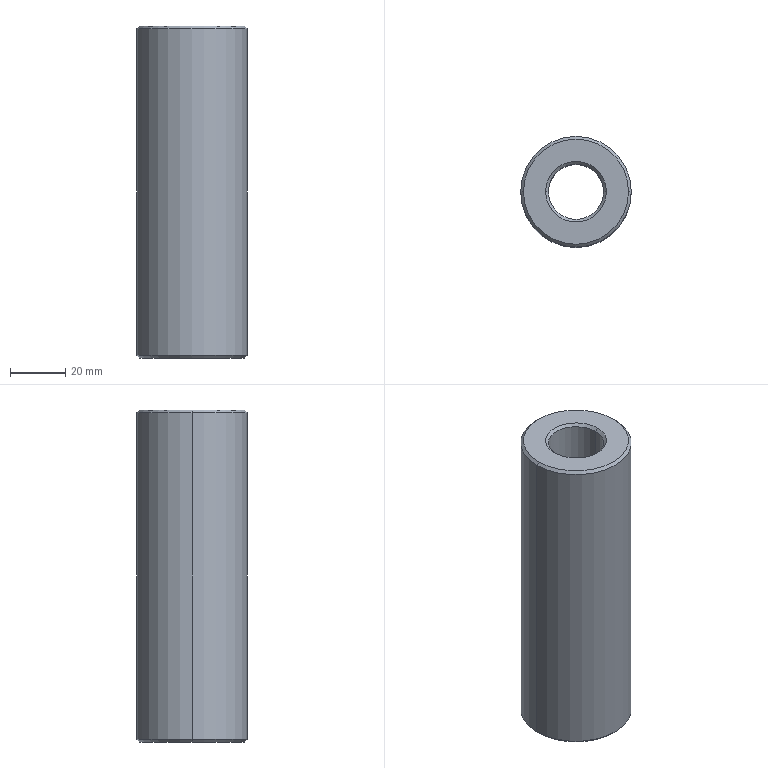Part | STEP file | BCC3 H14_7 | 1 solid | 14 faces | box 40 x 40 x 120 mm | volume 112909 mm3 | cone 8 | cylinder 4 | plane 2 | commonest cylinder face diameters 20 x2 40 x2
STEP:
#1=CARTESIAN_POINT('',(0.,0.,0.));
#2=DIRECTION('',(0.,0.,1.));
#3=DIRECTION('',(1.,0.,0.));
#4=AXIS2_PLACEMENT_3D('',#1,#2,#3);
#5=CARTESIAN_POINT('',(10.,0.,59.));
#6=VERTEX_POINT('',#5);
#7=CARTESIAN_POINT('',(11.,0.,60.));
#8=VERTEX_POINT('',#7);
#9=CARTESIAN_POINT('',(10.,0.,59.));
#10=DIRECTION('',(0.7071,0.,0.7071));
#11=VECTOR('',#10,1.);
#12=LINE('',#9,#11);
#13=CARTESIAN_POINT('',(0.,0.,59.));
#14=DIRECTION('',(0.,0.,1.));
#15=DIRECTION('',(1.,0.,0.));
#16=AXIS2_PLACEMENT_3D('',#13,#14,#15);
#17=CONICAL_SURFACE('',#16,10.,0.7854);
#18=CARTESIAN_POINT('',(6.283,0.));
#19=DIRECTION('',(0.,1.));
#20=VECTOR('',#19,1.);
#21=LINE('',#18,#20);
#22=(GEOMETRIC_REPRESENTATION_CONTEXT(2)PARAMETRIC_REPRESENTATION_CONTEXT()REPRESENTATION_CONTEXT('',''));
#23=DEFINITIONAL_REPRESENTATION('',(#21),#22);
#24=PCURVE('',#17,#23);
#25=CARTESIAN_POINT('',(0.,0.,59.));
#26=DIRECTION('',(0.,0.,1.));
#27=DIRECTION('',(1.,0.,0.));
#28=AXIS2_PLACEMENT_3D('',#25,#26,#27);
#29=CONICAL_SURFACE('',#28,10.,0.7854);
#30=CARTESIAN_POINT('',(0.,0.));
#31=DIRECTION('',(0.,1.));
#32=VECTOR('',#31,1.);
#33=LINE('',#30,#32);
#34=(GEOMETRIC_REPRESENTATION_CONTEXT(2)PARAMETRIC_REPRESENTATION_CONTEXT()REPRESENTATION_CONTEXT('',''));
#35=DEFINITIONAL_REPRESENTATION('',(#33),#34);
#36=PCURVE('',#29,#35);
#37=SURFACE_CURVE('',#12,(#24,#36),.PCURVE_S1.);
#38=EDGE_CURVE('',#6,#8,#37,.T.);
#39=ORIENTED_EDGE('',*,*,#38,.T.);
#40=CARTESIAN_POINT('',(-11.,0.,60.));
#41=VERTEX_POINT('',#40);
#42=CARTESIAN_POINT('',(0.,0.,60.));
#43=DIRECTION('',(0.,0.,-1.));
#44=DIRECTION('',(1.,0.,0.));
#45=AXIS2_PLACEMENT_3D('',#42,#43,#44);
#46=CIRCLE('',#45,11.);
#47=CARTESIAN_POINT('',(6.283,1.));
#48=DIRECTION('',(-1.,0.));
#49=VECTOR('',#48,1.);
#50=LINE('',#47,#49);
#51=(GEOMETRIC_REPRESENTATION_CONTEXT(2)PARAMETRIC_REPRESENTATION_CONTEXT()REPRESENTATION_CONTEXT('',''));
#52=DEFINITIONAL_REPRESENTATION('',(#50),#51);
#53=PCURVE('',#17,#52);
#54=CARTESIAN_POINT('',(0.,0.,60.));
#55=DIRECTION('',(0.,0.,1.));
#56=DIRECTION('',(1.,0.,0.));
#57=AXIS2_PLACEMENT_3D('',#54,#55,#56);
#58=PLANE('',#57);
#59=CARTESIAN_POINT('',(11.,0.));
#60=CARTESIAN_POINT('',(11.,-19.053));
#61=CARTESIAN_POINT('',(-5.5,-9.526));
#62=CARTESIAN_POINT('',(-22.,0.));
#63=CARTESIAN_POINT('',(-5.5,9.526));
#64=CARTESIAN_POINT('',(11.,19.053));
#65=CARTESIAN_POINT('',(11.,0.));
#66=(BOUNDED_CURVE()B_SPLINE_CURVE(2,(#59,#60,#61,#62,#63,#64,#65),.UNSPECIFIED.,.T.,.F.)B_SPLINE_CURVE_WITH_KNOTS((1,2,2,2,2,1),(-2.094,0.,2.094,4.189,6.283,8.378),.UNSPECIFIED.)CURVE()GEOMETRIC_REPRESENTATION_ITEM()RATIONAL_B_SPLINE_CURVE((1.,0.5,1.,0.5,1.,0.5,1.))REPRESENTATION_ITEM(''));
#67=(GEOMETRIC_REPRESENTATION_CONTEXT(2)PARAMETRIC_REPRESENTATION_CONTEXT()REPRESENTATION_CONTEXT('',''));
#68=DEFINITIONAL_REPRESENTATION('',(#66),#67);
#69=PCURVE('',#58,#68);
#70=SURFACE_CURVE('',#46,(#53,#69),.PCURVE_S1.);
#71=EDGE_CURVE('',#8,#41,#70,.T.);
#72=ORIENTED_EDGE('',*,*,#71,.T.);
#73=CARTESIAN_POINT('',(-10.,0.,59.));
#74=VERTEX_POINT('',#73);
#75=CARTESIAN_POINT('',(-10.,0.,59.));
#76=DIRECTION('',(-0.7071,0.,0.7071));
#77=VECTOR('',#76,1.);
#78=LINE('',#75,#77);
#79=CARTESIAN_POINT('',(3.142,0.));
#80=DIRECTION('',(0.,1.));
#81=VECTOR('',#80,1.);
#82=LINE('',#79,#81);
#83=(GEOMETRIC_REPRESENTATION_CONTEXT(2)PARAMETRIC_REPRESENTATION_CONTEXT()REPRESENTATION_CONTEXT('',''));
#84=DEFINITIONAL_REPRESENTATION('',(#82),#83);
#85=PCURVE('',#17,#84);
#86=CARTESIAN_POINT('',(3.142,0.));
#87=DIRECTION('',(0.,1.));
#88=VECTOR('',#87,1.);
#89=LINE('',#86,#88);
#90=(GEOMETRIC_REPRESENTATION_CONTEXT(2)PARAMETRIC_REPRESENTATION_CONTEXT()REPRESENTATION_CONTEXT('',''));
#91=DEFINITIONAL_REPRESENTATION('',(#89),#90);
#92=PCURVE('',#29,#91);
#93=SURFACE_CURVE('',#78,(#85,#92),.PCURVE_S1.);
#94=EDGE_CURVE('',#74,#41,#93,.T.);
#95=ORIENTED_EDGE('',*,*,#94,.F.);
#96=CARTESIAN_POINT('',(0.,0.,59.));
#97=DIRECTION('',(0.,0.,1.));
#98=DIRECTION('',(1.,0.,0.));
#99=AXIS2_PLACEMENT_3D('',#96,#97,#98);
#100=CIRCLE('',#99,10.);
#101=CARTESIAN_POINT('',(0.,0.));
#102=DIRECTION('',(1.,0.));
#103=VECTOR('',#102,1.);
#104=LINE('',#101,#103);
#105=(GEOMETRIC_REPRESENTATION_CONTEXT(2)PARAMETRIC_REPRESENTATION_CONTEXT()REPRESENTATION_CONTEXT('',''));
#106=DEFINITIONAL_REPRESENTATION('',(#104),#105);
#107=PCURVE('',#17,#106);
#108=CARTESIAN_POINT('',(0.,0.,60.));
#109=DIRECTION('',(0.,0.,-1.));
#110=DIRECTION('',(-1.,0.,0.));
#111=AXIS2_PLACEMENT_3D('',#108,#109,#110);
#112=CYLINDRICAL_SURFACE('',#111,10.);
#113=CARTESIAN_POINT('',(9.425,1.));
#114=DIRECTION('',(-1.,0.));
#115=VECTOR('',#114,1.);
#116=LINE('',#113,#115);
#117=(GEOMETRIC_REPRESENTATION_CONTEXT(2)PARAMETRIC_REPRESENTATION_CONTEXT()REPRESENTATION_CONTEXT('',''));
#118=DEFINITIONAL_REPRESENTATION('',(#116),#117);
#119=PCURVE('',#112,#118);
#120=SURFACE_CURVE('',#100,(#107,#119),.PCURVE_S1.);
#121=EDGE_CURVE('',#74,#6,#120,.T.);
#122=ORIENTED_EDGE('',*,*,#121,.T.);
#123=EDGE_LOOP('',(#39,#72,#95,#122));
#124=FACE_BOUND('',#123,.F.);
#125=ADVANCED_FACE('',(#124),#17,.F.);
#126=CARTESIAN_POINT('',(19.,0.,60.));
#127=VERTEX_POINT('',#126);
#128=CARTESIAN_POINT('',(-19.,0.,60.));
#129=VERTEX_POINT('',#128);
#130=CARTESIAN_POINT('',(0.,0.,60.));
#131=DIRECTION('',(0.,0.,1.));
#132=DIRECTION('',(1.,0.,0.));
#133=AXIS2_PLACEMENT_3D('',#130,#131,#132);
#134=CIRCLE('',#133,19.);
#135=CARTESIAN_POINT('',(0.,0.,60.));
#136=DIRECTION('',(0.,0.,-1.));
#137=DIRECTION('',(-1.,0.,0.));
#138=AXIS2_PLACEMENT_3D('',#135,#136,#137);
#139=CONICAL_SURFACE('',#138,19.,0.7854);
#140=CARTESIAN_POINT('',(3.142,0.));
#141=DIRECTION('',(-1.,0.));
#142=VECTOR('',#141,1.);
#143=LINE('',#140,#142);
#144=(GEOMETRIC_REPRESENTATION_CONTEXT(2)PARAMETRIC_REPRESENTATION_CONTEXT()REPRESENTATION_CONTEXT('',''));
#145=DEFINITIONAL_REPRESENTATION('',(#143),#144);
#146=PCURVE('',#139,#145);
#147=CARTESIAN_POINT('',(0.,0.));
#148=DIRECTION('',(1.,0.));
#149=AXIS2_PLACEMENT_2D('',#147,#148);
#150=CIRCLE('',#149,19.);
#151=(GEOMETRIC_REPRESENTATION_CONTEXT(2)PARAMETRIC_REPRESENTATION_CONTEXT()REPRESENTATION_CONTEXT('',''));
#152=DEFINITIONAL_REPRESENTATION('',(#150),#151);
#153=PCURVE('',#58,#152);
#154=SURFACE_CURVE('',#134,(#146,#153),.PCURVE_S1.);
#155=EDGE_CURVE('',#127,#129,#154,.T.);
#156=ORIENTED_EDGE('',*,*,#155,.F.);
#157=CARTESIAN_POINT('',(20.,0.,59.));
#158=VERTEX_POINT('',#157);
#159=CARTESIAN_POINT('',(19.,0.,60.));
#160=DIRECTION('',(0.7071,0.,-0.7071));
#161=VECTOR('',#160,1.);
#162=LINE('',#159,#161);
#163=CARTESIAN_POINT('',(3.142,0.));
#164=DIRECTION('',(0.,1.));
#165=VECTOR('',#164,1.);
#166=LINE('',#163,#165);
#167=(GEOMETRIC_REPRESENTATION_CONTEXT(2)PARAMETRIC_REPRESENTATION_CONTEXT()REPRESENTATION_CONTEXT('',''));
#168=DEFINITIONAL_REPRESENTATION('',(#166),#167);
#169=PCURVE('',#139,#168);
#170=CARTESIAN_POINT('',(0.,0.,60.));
#171=DIRECTION('',(0.,0.,-1.));
#172=DIRECTION('',(-1.,0.,0.));
#173=AXIS2_PLACEMENT_3D('',#170,#171,#172);
#174=CONICAL_SURFACE('',#173,19.,0.7854);
#175=CARTESIAN_POINT('',(3.142,0.));
#176=DIRECTION('',(0.,1.));
#177=VECTOR('',#176,1.);
#178=LINE('',#175,#177);
#179=(GEOMETRIC_REPRESENTATION_CONTEXT(2)PARAMETRIC_REPRESENTATION_CONTEXT()REPRESENTATION_CONTEXT('',''));
#180=DEFINITIONAL_REPRESENTATION('',(#178),#179);
#181=PCURVE('',#174,#180);
#182=SURFACE_CURVE('',#162,(#169,#181),.PCURVE_S1.);
#183=EDGE_CURVE('',#127,#158,#182,.T.);
#184=ORIENTED_EDGE('',*,*,#183,.T.);
#185=CARTESIAN_POINT('',(-20.,0.,59.));
#186=VERTEX_POINT('',#185);
#187=CARTESIAN_POINT('',(0.,0.,59.));
#188=DIRECTION('',(0.,0.,-1.));
#189=DIRECTION('',(1.,0.,0.));
#190=AXIS2_PLACEMENT_3D('',#187,#188,#189);
#191=CIRCLE('',#190,20.);
#192=CARTESIAN_POINT('',(-3.142,1.));
#193=DIRECTION('',(1.,0.));
#194=VECTOR('',#193,1.);
#195=LINE('',#192,#194);
#196=(GEOMETRIC_REPRESENTATION_CONTEXT(2)PARAMETRIC_REPRESENTATION_CONTEXT()REPRESENTATION_CONTEXT('',''));
#197=DEFINITIONAL_REPRESENTATION('',(#195),#196);
#198=PCURVE('',#139,#197);
#199=CARTESIAN_POINT('',(0.,0.,60.));
#200=DIRECTION('',(0.,0.,-1.));
#201=DIRECTION('',(-1.,0.,0.));
#202=AXIS2_PLACEMENT_3D('',#199,#200,#201);
#203=CYLINDRICAL_SURFACE('',#202,20.);
#204=CARTESIAN_POINT('',(-3.142,1.));
#205=DIRECTION('',(1.,0.));
#206=VECTOR('',#205,1.);
#207=LINE('',#204,#206);
#208=(GEOMETRIC_REPRESENTATION_CONTEXT(2)PARAMETRIC_REPRESENTATION_CONTEXT()REPRESENTATION_CONTEXT('',''));
#209=DEFINITIONAL_REPRESENTATION('',(#207),#208);
#210=PCURVE('',#203,#209);
#211=SURFACE_CURVE('',#191,(#198,#210),.PCURVE_S1.);
#212=EDGE_CURVE('',#186,#158,#211,.T.);
#213=ORIENTED_EDGE('',*,*,#212,.F.);
#214=CARTESIAN_POINT('',(-19.,0.,60.));
#215=DIRECTION('',(-0.7071,0.,-0.7071));
#216=VECTOR('',#215,1.);
#217=LINE('',#214,#216);
#218=CARTESIAN_POINT('',(0.,0.));
#219=DIRECTION('',(0.,1.));
#220=VECTOR('',#219,1.);
#221=LINE('',#218,#220);
#222=(GEOMETRIC_REPRESENTATION_CONTEXT(2)PARAMETRIC_REPRESENTATION_CONTEXT()REPRESENTATION_CONTEXT('',''));
#223=DEFINITIONAL_REPRESENTATION('',(#221),#222);
#224=PCURVE('',#139,#223);
#225=CARTESIAN_POINT('',(6.283,0.));
#226=DIRECTION('',(0.,1.));
#227=VECTOR('',#226,1.);
#228=LINE('',#225,#227);
#229=(GEOMETRIC_REPRESENTATION_CONTEXT(2)PARAMETRIC_REPRESENTATION_CONTEXT()REPRESENTATION_CONTEXT('',''));
#230=DEFINITIONAL_REPRESENTATION('',(#228),#229);
#231=PCURVE('',#174,#230);
#232=SURFACE_CURVE('',#217,(#224,#231),.PCURVE_S1.);
#233=EDGE_CURVE('',#129,#186,#232,.T.);
#234=ORIENTED_EDGE('',*,*,#233,.F.);
#235=EDGE_LOOP('',(#156,#184,#213,#234));
#236=FACE_BOUND('',#235,.T.);
#237=ADVANCED_FACE('',(#236),#139,.T.);
#238=CARTESIAN_POINT('',(-10.,0.,-59.));
#239=VERTEX_POINT('',#238);
#240=CARTESIAN_POINT('',(-11.,0.,-60.));
#241=VERTEX_POINT('',#240);
#242=CARTESIAN_POINT('',(-11.,0.,-60.));
#243=DIRECTION('',(-0.7071,0.,-0.7071));
#244=VECTOR('',#243,1.);
#245=LINE('',#242,#244);
#246=CARTESIAN_POINT('',(0.,0.,-60.));
#247=DIRECTION('',(0.,0.,-1.));
#248=DIRECTION('',(-1.,0.,0.));
#249=AXIS2_PLACEMENT_3D('',#246,#247,#248);
#250=CONICAL_SURFACE('',#249,11.,0.7854);
#251=CARTESIAN_POINT('',(6.283,0.));
#252=DIRECTION('',(0.,1.));
#253=VECTOR('',#252,1.);
#254=LINE('',#251,#253);
#255=(GEOMETRIC_REPRESENTATION_CONTEXT(2)PARAMETRIC_REPRESENTATION_CONTEXT()REPRESENTATION_CONTEXT('',''));
#256=DEFINITIONAL_REPRESENTATION('',(#254),#255);
#257=PCURVE('',#250,#256);
#258=CARTESIAN_POINT('',(0.,0.,-60.));
#259=DIRECTION('',(0.,0.,-1.));
#260=DIRECTION('',(-1.,0.,0.));
#261=AXIS2_PLACEMENT_3D('',#258,#259,#260);
#262=CONICAL_SURFACE('',#261,11.,0.7854);
#263=CARTESIAN_POINT('',(0.,0.));
#264=DIRECTION('',(0.,1.));
#265=VECTOR('',#264,1.);
#266=LINE('',#263,#265);
#267=(GEOMETRIC_REPRESENTATION_CONTEXT(2)PARAMETRIC_REPRESENTATION_CONTEXT()REPRESENTATION_CONTEXT('',''));
#268=DEFINITIONAL_REPRESENTATION('',(#266),#267);
#269=PCURVE('',#262,#268);
#270=SURFACE_CURVE('',#245,(#257,#269),.PCURVE_S1.);
#271=EDGE_CURVE('',#239,#241,#270,.T.);
#272=ORIENTED_EDGE('',*,*,#271,.T.);
#273=CARTESIAN_POINT('',(11.,0.,-60.));
#274=VERTEX_POINT('',#273);
#275=CARTESIAN_POINT('',(0.,0.,-60.));
#276=DIRECTION('',(0.,0.,1.));
#277=DIRECTION('',(1.,0.,0.));
#278=AXIS2_PLACEMENT_3D('',#275,#276,#277);
#279=CIRCLE('',#278,11.);
#280=CARTESIAN_POINT('',(9.425,0.));
#281=DIRECTION('',(-1.,0.));
#282=VECTOR('',#281,1.);
#283=LINE('',#280,#282);
#284=(GEOMETRIC_REPRESENTATION_CONTEXT(2)PARAMETRIC_REPRESENTATION_CONTEXT()REPRESENTATION_CONTEXT('',''));
#285=DEFINITIONAL_REPRESENTATION('',(#283),#284);
#286=PCURVE('',#250,#285);
#287=CARTESIAN_POINT('',(0.,0.,-60.));
#288=DIRECTION('',(0.,0.,1.));
#289=DIRECTION('',(1.,0.,0.));
#290=AXIS2_PLACEMENT_3D('',#287,#288,#289);
#291=PLANE('',#290);
#292=CARTESIAN_POINT('',(0.,0.));
#293=DIRECTION('',(1.,0.));
#294=AXIS2_PLACEMENT_2D('',#292,#293);
#295=CIRCLE('',#294,11.);
#296=(GEOMETRIC_REPRESENTATION_CONTEXT(2)PARAMETRIC_REPRESENTATION_CONTEXT()REPRESENTATION_CONTEXT('',''));
#297=DEFINITIONAL_REPRESENTATION('',(#295),#296);
#298=PCURVE('',#291,#297);
#299=SURFACE_CURVE('',#279,(#286,#298),.PCURVE_S1.);
#300=EDGE_CURVE('',#241,#274,#299,.T.);
#301=ORIENTED_EDGE('',*,*,#300,.T.);
#302=CARTESIAN_POINT('',(10.,0.,-59.));
#303=VERTEX_POINT('',#302);
#304=CARTESIAN_POINT('',(11.,0.,-60.));
#305=DIRECTION('',(0.7071,0.,-0.7071));
#306=VECTOR('',#305,1.);
#307=LINE('',#304,#306);
#308=CARTESIAN_POINT('',(3.142,0.));
#309=DIRECTION('',(0.,1.));
#310=VECTOR('',#309,1.);
#311=LINE('',#308,#310);
#312=(GEOMETRIC_REPRESENTATION_CONTEXT(2)PARAMETRIC_REPRESENTATION_CONTEXT()REPRESENTATION_CONTEXT('',''));
#313=DEFINITIONAL_REPRESENTATION('',(#311),#312);
#314=PCURVE('',#250,#313);
#315=CARTESIAN_POINT('',(3.142,0.));
#316=DIRECTION('',(0.,1.));
#317=VECTOR('',#316,1.);
#318=LINE('',#315,#317);
#319=(GEOMETRIC_REPRESENTATION_CONTEXT(2)PARAMETRIC_REPRESENTATION_CONTEXT()REPRESENTATION_CONTEXT('',''));
#320=DEFINITIONAL_REPRESENTATION('',(#318),#319);
#321=PCURVE('',#262,#320);
#322=SURFACE_CURVE('',#307,(#314,#321),.PCURVE_S1.);
#323=EDGE_CURVE('',#303,#274,#322,.T.);
#324=ORIENTED_EDGE('',*,*,#323,.F.);
#325=CARTESIAN_POINT('',(0.,0.,-59.));
#326=DIRECTION('',(0.,0.,-1.));
#327=DIRECTION('',(1.,0.,0.));
#328=AXIS2_PLACEMENT_3D('',#325,#326,#327);
#329=CIRCLE('',#328,10.);
#330=CARTESIAN_POINT('',(3.142,-1.));
#331=DIRECTION('',(1.,0.));
#332=VECTOR('',#331,1.);
#333=LINE('',#330,#332);
#334=(GEOMETRIC_REPRESENTATION_CONTEXT(2)PARAMETRIC_REPRESENTATION_CONTEXT()REPRESENTATION_CONTEXT('',''));
#335=DEFINITIONAL_REPRESENTATION('',(#333),#334);
#336=PCURVE('',#250,#335);
#337=CARTESIAN_POINT('',(3.142,119.));
#338=DIRECTION('',(1.,0.));
#339=VECTOR('',#338,1.);
#340=LINE('',#337,#339);
#341=(GEOMETRIC_REPRESENTATION_CONTEXT(2)PARAMETRIC_REPRESENTATION_CONTEXT()REPRESENTATION_CONTEXT('',''));
#342=DEFINITIONAL_REPRESENTATION('',(#340),#341);
#343=PCURVE('',#112,#342);
#344=SURFACE_CURVE('',#329,(#336,#343),.PCURVE_S1.);
#345=EDGE_CURVE('',#303,#239,#344,.T.);
#346=ORIENTED_EDGE('',*,*,#345,.T.);
#347=EDGE_LOOP('',(#272,#301,#324,#346));
#348=FACE_BOUND('',#347,.F.);
#349=ADVANCED_FACE('',(#348),#250,.F.);
#350=CARTESIAN_POINT('',(-19.,0.,-60.));
#351=VERTEX_POINT('',#350);
#352=CARTESIAN_POINT('',(19.,0.,-60.));
#353=VERTEX_POINT('',#352);
#354=CARTESIAN_POINT('',(0.,0.,-60.));
#355=DIRECTION('',(0.,0.,-1.));
#356=DIRECTION('',(1.,0.,0.));
#357=AXIS2_PLACEMENT_3D('',#354,#355,#356);
#358=CIRCLE('',#357,19.);
#359=CARTESIAN_POINT('',(0.,0.,-59.));
#360=DIRECTION('',(0.,0.,1.));
#361=DIRECTION('',(1.,0.,0.));
#362=AXIS2_PLACEMENT_3D('',#359,#360,#361);
#363=CONICAL_SURFACE('',#362,20.,0.7854);
#364=CARTESIAN_POINT('',(6.283,-1.));
#365=DIRECTION('',(-1.,0.));
#366=VECTOR('',#365,1.);
#367=LINE('',#364,#366);
#368=(GEOMETRIC_REPRESENTATION_CONTEXT(2)PARAMETRIC_REPRESENTATION_CONTEXT()REPRESENTATION_CONTEXT('',''));
#369=DEFINITIONAL_REPRESENTATION('',(#367),#368);
#370=PCURVE('',#363,#369);
#371=CARTESIAN_POINT('',(19.,0.));
#372=CARTESIAN_POINT('',(19.,-32.909));
#373=CARTESIAN_POINT('',(-9.5,-16.454));
#374=CARTESIAN_POINT('',(-38.,0.));
#375=CARTESIAN_POINT('',(-9.5,16.454));
#376=CARTESIAN_POINT('',(19.,32.909));
#377=CARTESIAN_POINT('',(19.,0.));
#378=(BOUNDED_CURVE()B_SPLINE_CURVE(2,(#371,#372,#373,#374,#375,#376,#377),.UNSPECIFIED.,.T.,.F.)B_SPLINE_CURVE_WITH_KNOTS((1,2,2,2,2,1),(-2.094,0.,2.094,4.189,6.283,8.378),.UNSPECIFIED.)CURVE()GEOMETRIC_REPRESENTATION_ITEM()RATIONAL_B_SPLINE_CURVE((1.,0.5,1.,0.5,1.,0.5,1.))REPRESENTATION_ITEM(''));
#379=(GEOMETRIC_REPRESENTATION_CONTEXT(2)PARAMETRIC_REPRESENTATION_CONTEXT()REPRESENTATION_CONTEXT('',''));
#380=DEFINITIONAL_REPRESENTATION('',(#378),#379);
#381=PCURVE('',#291,#380);
#382=SURFACE_CURVE('',#358,(#370,#381),.PCURVE_S1.);
#383=EDGE_CURVE('',#351,#353,#382,.T.);
#384=ORIENTED_EDGE('',*,*,#383,.F.);
#385=CARTESIAN_POINT('',(-20.,0.,-59.));
#386=VERTEX_POINT('',#385);
#387=CARTESIAN_POINT('',(-20.,0.,-59.));
#388=DIRECTION('',(-0.7071,0.,0.7071));
#389=VECTOR('',#388,1.);
#390=LINE('',#387,#389);
#391=CARTESIAN_POINT('',(3.142,0.));
#392=DIRECTION('',(0.,1.));
#393=VECTOR('',#392,1.);
#394=LINE('',#391,#393);
#395=(GEOMETRIC_REPRESENTATION_CONTEXT(2)PARAMETRIC_REPRESENTATION_CONTEXT()REPRESENTATION_CONTEXT('',''));
#396=DEFINITIONAL_REPRESENTATION('',(#394),#395);
#397=PCURVE('',#363,#396);
#398=CARTESIAN_POINT('',(0.,0.,-59.));
#399=DIRECTION('',(0.,0.,1.));
#400=DIRECTION('',(1.,0.,0.));
#401=AXIS2_PLACEMENT_3D('',#398,#399,#400);
#402=CONICAL_SURFACE('',#401,20.,0.7854);
#403=CARTESIAN_POINT('',(3.142,0.));
#404=DIRECTION('',(0.,1.));
#405=VECTOR('',#404,1.);
#406=LINE('',#403,#405);
#407=(GEOMETRIC_REPRESENTATION_CONTEXT(2)PARAMETRIC_REPRESENTATION_CONTEXT()REPRESENTATION_CONTEXT('',''));
#408=DEFINITIONAL_REPRESENTATION('',(#406),#407);
#409=PCURVE('',#402,#408);
#410=SURFACE_CURVE('',#390,(#397,#409),.PCURVE_S1.);
#411=EDGE_CURVE('',#351,#386,#410,.T.);
#412=ORIENTED_EDGE('',*,*,#411,.T.);
#413=CARTESIAN_POINT('',(20.,0.,-59.));
#414=VERTEX_POINT('',#413);
#415=CARTESIAN_POINT('',(0.,0.,-59.));
#416=DIRECTION('',(0.,0.,1.));
#417=DIRECTION('',(1.,0.,0.));
#418=AXIS2_PLACEMENT_3D('',#415,#416,#417);
#419=CIRCLE('',#418,20.);
#420=CARTESIAN_POINT('',(0.,0.));
#421=DIRECTION('',(1.,0.));
#422=VECTOR('',#421,1.);
#423=LINE('',#420,#422);
#424=(GEOMETRIC_REPRESENTATION_CONTEXT(2)PARAMETRIC_REPRESENTATION_CONTEXT()REPRESENTATION_CONTEXT('',''));
#425=DEFINITIONAL_REPRESENTATION('',(#423),#424);
#426=PCURVE('',#363,#425);
#427=CARTESIAN_POINT('',(3.142,119.));
#428=DIRECTION('',(-1.,0.));
#429=VECTOR('',#428,1.);
#430=LINE('',#427,#429);
#431=(GEOMETRIC_REPRESENTATION_CONTEXT(2)PARAMETRIC_REPRESENTATION_CONTEXT()REPRESENTATION_CONTEXT('',''));
#432=DEFINITIONAL_REPRESENTATION('',(#430),#431);
#433=PCURVE('',#203,#432);
#434=SURFACE_CURVE('',#419,(#426,#433),.PCURVE_S1.);
#435=EDGE_CURVE('',#414,#386,#434,.T.);
#436=ORIENTED_EDGE('',*,*,#435,.F.);
#437=CARTESIAN_POINT('',(20.,0.,-59.));
#438=DIRECTION('',(0.7071,0.,0.7071));
#439=VECTOR('',#438,1.);
#440=LINE('',#437,#439);
#441=CARTESIAN_POINT('',(0.,0.));
#442=DIRECTION('',(0.,1.));
#443=VECTOR('',#442,1.);
#444=LINE('',#441,#443);
#445=(GEOMETRIC_REPRESENTATION_CONTEXT(2)PARAMETRIC_REPRESENTATION_CONTEXT()REPRESENTATION_CONTEXT('',''));
#446=DEFINITIONAL_REPRESENTATION('',(#444),#445);
#447=PCURVE('',#363,#446);
#448=CARTESIAN_POINT('',(6.283,0.));
#449=DIRECTION('',(0.,1.));
#450=VECTOR('',#449,1.);
#451=LINE('',#448,#450);
#452=(GEOMETRIC_REPRESENTATION_CONTEXT(2)PARAMETRIC_REPRESENTATION_CONTEXT()REPRESENTATION_CONTEXT('',''));
#453=DEFINITIONAL_REPRESENTATION('',(#451),#452);
#454=PCURVE('',#402,#453);
#455=SURFACE_CURVE('',#440,(#447,#454),.PCURVE_S1.);
#456=EDGE_CURVE('',#353,#414,#455,.T.);
#457=ORIENTED_EDGE('',*,*,#456,.F.);
#458=EDGE_LOOP('',(#384,#412,#436,#457));
#459=FACE_BOUND('',#458,.T.);
#460=ADVANCED_FACE('',(#459),#363,.T.);
#461=CARTESIAN_POINT('',(-10.,0.,60.));
#462=DIRECTION('',(0.,0.,-1.));
#463=VECTOR('',#462,1.);
#464=LINE('',#461,#463);
#465=CARTESIAN_POINT('',(6.283,0.));
#466=DIRECTION('',(0.,1.));
#467=VECTOR('',#466,1.);
#468=LINE('',#465,#467);
#469=(GEOMETRIC_REPRESENTATION_CONTEXT(2)PARAMETRIC_REPRESENTATION_CONTEXT()REPRESENTATION_CONTEXT('',''));
#470=DEFINITIONAL_REPRESENTATION('',(#468),#469);
#471=PCURVE('',#112,#470);
#472=CARTESIAN_POINT('',(0.,0.,60.));
#473=DIRECTION('',(0.,0.,-1.));
#474=DIRECTION('',(-1.,0.,0.));
#475=AXIS2_PLACEMENT_3D('',#472,#473,#474);
#476=CYLINDRICAL_SURFACE('',#475,10.);
#477=CARTESIAN_POINT('',(0.,0.));
#478=DIRECTION('',(0.,1.));
#479=VECTOR('',#478,1.);
#480=LINE('',#477,#479);
#481=(GEOMETRIC_REPRESENTATION_CONTEXT(2)PARAMETRIC_REPRESENTATION_CONTEXT()REPRESENTATION_CONTEXT('',''));
#482=DEFINITIONAL_REPRESENTATION('',(#480),#481);
#483=PCURVE('',#476,#482);
#484=SURFACE_CURVE('',#464,(#471,#483),.PCURVE_S1.);
#485=EDGE_CURVE('',#74,#239,#484,.T.);
#486=ORIENTED_EDGE('',*,*,#485,.T.);
#487=ORIENTED_EDGE('',*,*,#345,.F.);
#488=CARTESIAN_POINT('',(10.,0.,60.));
#489=DIRECTION('',(0.,0.,-1.));
#490=VECTOR('',#489,1.);
#491=LINE('',#488,#490);
#492=CARTESIAN_POINT('',(3.142,0.));
#493=DIRECTION('',(0.,1.));
#494=VECTOR('',#493,1.);
#495=LINE('',#492,#494);
#496=(GEOMETRIC_REPRESENTATION_CONTEXT(2)PARAMETRIC_REPRESENTATION_CONTEXT()REPRESENTATION_CONTEXT('',''));
#497=DEFINITIONAL_REPRESENTATION('',(#495),#496);
#498=PCURVE('',#112,#497);
#499=CARTESIAN_POINT('',(3.142,0.));
#500=DIRECTION('',(0.,1.));
#501=VECTOR('',#500,1.);
#502=LINE('',#499,#501);
#503=(GEOMETRIC_REPRESENTATION_CONTEXT(2)PARAMETRIC_REPRESENTATION_CONTEXT()REPRESENTATION_CONTEXT('',''));
#504=DEFINITIONAL_REPRESENTATION('',(#502),#503);
#505=PCURVE('',#476,#504);
#506=SURFACE_CURVE('',#491,(#498,#505),.PCURVE_S1.);
#507=EDGE_CURVE('',#6,#303,#506,.T.);
#508=ORIENTED_EDGE('',*,*,#507,.F.);
#509=ORIENTED_EDGE('',*,*,#121,.F.);
#510=EDGE_LOOP('',(#486,#487,#508,#509));
#511=FACE_BOUND('',#510,.F.);
#512=ADVANCED_FACE('',(#511),#112,.F.);
#513=ORIENTED_EDGE('',*,*,#212,.T.);
#514=CARTESIAN_POINT('',(20.,0.,60.));
#515=DIRECTION('',(0.,0.,-1.));
#516=VECTOR('',#515,1.);
#517=LINE('',#514,#516);
#518=CARTESIAN_POINT('',(3.142,0.));
#519=DIRECTION('',(0.,1.));
#520=VECTOR('',#519,1.);
#521=LINE('',#518,#520);
#522=(GEOMETRIC_REPRESENTATION_CONTEXT(2)PARAMETRIC_REPRESENTATION_CONTEXT()REPRESENTATION_CONTEXT('',''));
#523=DEFINITIONAL_REPRESENTATION('',(#521),#522);
#524=PCURVE('',#203,#523);
#525=CARTESIAN_POINT('',(0.,0.,60.));
#526=DIRECTION('',(0.,0.,-1.));
#527=DIRECTION('',(-1.,0.,0.));
#528=AXIS2_PLACEMENT_3D('',#525,#526,#527);
#529=CYLINDRICAL_SURFACE('',#528,20.);
#530=CARTESIAN_POINT('',(3.142,0.));
#531=DIRECTION('',(0.,1.));
#532=VECTOR('',#531,1.);
#533=LINE('',#530,#532);
#534=(GEOMETRIC_REPRESENTATION_CONTEXT(2)PARAMETRIC_REPRESENTATION_CONTEXT()REPRESENTATION_CONTEXT('',''));
#535=DEFINITIONAL_REPRESENTATION('',(#533),#534);
#536=PCURVE('',#529,#535);
#537=SURFACE_CURVE('',#517,(#524,#536),.PCURVE_S1.);
#538=EDGE_CURVE('',#158,#414,#537,.T.);
#539=ORIENTED_EDGE('',*,*,#538,.T.);
#540=ORIENTED_EDGE('',*,*,#435,.T.);
#541=CARTESIAN_POINT('',(-20.,0.,60.));
#542=DIRECTION('',(0.,0.,-1.));
#543=VECTOR('',#542,1.);
#544=LINE('',#541,#543);
#545=CARTESIAN_POINT('',(0.,0.));
#546=DIRECTION('',(0.,1.));
#547=VECTOR('',#546,1.);
#548=LINE('',#545,#547);
#549=(GEOMETRIC_REPRESENTATION_CONTEXT(2)PARAMETRIC_REPRESENTATION_CONTEXT()REPRESENTATION_CONTEXT('',''));
#550=DEFINITIONAL_REPRESENTATION('',(#548),#549);
#551=PCURVE('',#203,#550);
#552=CARTESIAN_POINT('',(6.283,0.));
#553=DIRECTION('',(0.,1.));
#554=VECTOR('',#553,1.);
#555=LINE('',#552,#554);
#556=(GEOMETRIC_REPRESENTATION_CONTEXT(2)PARAMETRIC_REPRESENTATION_CONTEXT()REPRESENTATION_CONTEXT('',''));
#557=DEFINITIONAL_REPRESENTATION('',(#555),#556);
#558=PCURVE('',#529,#557);
#559=SURFACE_CURVE('',#544,(#551,#558),.PCURVE_S1.);
#560=EDGE_CURVE('',#186,#386,#559,.T.);
#561=ORIENTED_EDGE('',*,*,#560,.F.);
#562=EDGE_LOOP('',(#513,#539,#540,#561));
#563=FACE_BOUND('',#562,.T.);
#564=ADVANCED_FACE('',(#563),#203,.T.);
#565=CARTESIAN_POINT('',(0.,0.,60.));
#566=DIRECTION('',(0.,0.,1.));
#567=DIRECTION('',(1.,0.,0.));
#568=AXIS2_PLACEMENT_3D('',#565,#566,#567);
#569=CIRCLE('',#568,19.);
#570=CARTESIAN_POINT('',(0.,0.));
#571=DIRECTION('',(1.,0.));
#572=AXIS2_PLACEMENT_2D('',#570,#571);
#573=CIRCLE('',#572,19.);
#574=(GEOMETRIC_REPRESENTATION_CONTEXT(2)PARAMETRIC_REPRESENTATION_CONTEXT()REPRESENTATION_CONTEXT('',''));
#575=DEFINITIONAL_REPRESENTATION('',(#573),#574);
#576=PCURVE('',#58,#575);
#577=CARTESIAN_POINT('',(9.425,0.));
#578=DIRECTION('',(-1.,0.));
#579=VECTOR('',#578,1.);
#580=LINE('',#577,#579);
#581=(GEOMETRIC_REPRESENTATION_CONTEXT(2)PARAMETRIC_REPRESENTATION_CONTEXT()REPRESENTATION_CONTEXT('',''));
#582=DEFINITIONAL_REPRESENTATION('',(#580),#581);
#583=PCURVE('',#174,#582);
#584=SURFACE_CURVE('',#569,(#576,#583),.PCURVE_S1.);
#585=EDGE_CURVE('',#129,#127,#584,.T.);
#586=ORIENTED_EDGE('',*,*,#585,.T.);
#587=ORIENTED_EDGE('',*,*,#155,.T.);
#588=EDGE_LOOP('',(#586,#587));
#589=FACE_BOUND('',#588,.T.);
#590=ORIENTED_EDGE('',*,*,#71,.T.);
#591=CARTESIAN_POINT('',(0.,0.,60.));
#592=DIRECTION('',(0.,0.,-1.));
#593=DIRECTION('',(1.,0.,0.));
#594=AXIS2_PLACEMENT_3D('',#591,#592,#593);
#595=CIRCLE('',#594,11.);
#596=CARTESIAN_POINT('',(11.,0.));
#597=CARTESIAN_POINT('',(11.,-19.053));
#598=CARTESIAN_POINT('',(-5.5,-9.526));
#599=CARTESIAN_POINT('',(-22.,0.));
#600=CARTESIAN_POINT('',(-5.5,9.526));
#601=CARTESIAN_POINT('',(11.,19.053));
#602=CARTESIAN_POINT('',(11.,0.));
#603=(BOUNDED_CURVE()B_SPLINE_CURVE(2,(#596,#597,#598,#599,#600,#601,#602),.UNSPECIFIED.,.T.,.F.)B_SPLINE_CURVE_WITH_KNOTS((1,2,2,2,2,1),(-2.094,0.,2.094,4.189,6.283,8.378),.UNSPECIFIED.)CURVE()GEOMETRIC_REPRESENTATION_ITEM()RATIONAL_B_SPLINE_CURVE((1.,0.5,1.,0.5,1.,0.5,1.))REPRESENTATION_ITEM(''));
#604=(GEOMETRIC_REPRESENTATION_CONTEXT(2)PARAMETRIC_REPRESENTATION_CONTEXT()REPRESENTATION_CONTEXT('',''));
#605=DEFINITIONAL_REPRESENTATION('',(#603),#604);
#606=PCURVE('',#58,#605);
#607=CARTESIAN_POINT('',(6.283,1.));
#608=DIRECTION('',(-1.,0.));
#609=VECTOR('',#608,1.);
#610=LINE('',#607,#609);
#611=(GEOMETRIC_REPRESENTATION_CONTEXT(2)PARAMETRIC_REPRESENTATION_CONTEXT()REPRESENTATION_CONTEXT('',''));
#612=DEFINITIONAL_REPRESENTATION('',(#610),#611);
#613=PCURVE('',#29,#612);
#614=SURFACE_CURVE('',#595,(#606,#613),.PCURVE_S1.);
#615=EDGE_CURVE('',#41,#8,#614,.T.);
#616=ORIENTED_EDGE('',*,*,#615,.T.);
#617=EDGE_LOOP('',(#590,#616));
#618=FACE_BOUND('',#617,.T.);
#619=ADVANCED_FACE('',(#589,#618),#58,.T.);
#620=CARTESIAN_POINT('',(0.,0.,-60.));
#621=DIRECTION('',(0.,0.,-1.));
#622=DIRECTION('',(1.,0.,0.));
#623=AXIS2_PLACEMENT_3D('',#620,#621,#622);
#624=CIRCLE('',#623,19.);
#625=CARTESIAN_POINT('',(19.,0.));
#626=CARTESIAN_POINT('',(19.,-32.909));
#627=CARTESIAN_POINT('',(-9.5,-16.454));
#628=CARTESIAN_POINT('',(-38.,0.));
#629=CARTESIAN_POINT('',(-9.5,16.454));
#630=CARTESIAN_POINT('',(19.,32.909));
#631=CARTESIAN_POINT('',(19.,0.));
#632=(BOUNDED_CURVE()B_SPLINE_CURVE(2,(#625,#626,#627,#628,#629,#630,#631),.UNSPECIFIED.,.T.,.F.)B_SPLINE_CURVE_WITH_KNOTS((1,2,2,2,2,1),(-2.094,0.,2.094,4.189,6.283,8.378),.UNSPECIFIED.)CURVE()GEOMETRIC_REPRESENTATION_ITEM()RATIONAL_B_SPLINE_CURVE((1.,0.5,1.,0.5,1.,0.5,1.))REPRESENTATION_ITEM(''));
#633=(GEOMETRIC_REPRESENTATION_CONTEXT(2)PARAMETRIC_REPRESENTATION_CONTEXT()REPRESENTATION_CONTEXT('',''));
#634=DEFINITIONAL_REPRESENTATION('',(#632),#633);
#635=PCURVE('',#291,#634);
#636=CARTESIAN_POINT('',(6.283,-1.));
#637=DIRECTION('',(-1.,0.));
#638=VECTOR('',#637,1.);
#639=LINE('',#636,#638);
#640=(GEOMETRIC_REPRESENTATION_CONTEXT(2)PARAMETRIC_REPRESENTATION_CONTEXT()REPRESENTATION_CONTEXT('',''));
#641=DEFINITIONAL_REPRESENTATION('',(#639),#640);
#642=PCURVE('',#402,#641);
#643=SURFACE_CURVE('',#624,(#635,#642),.PCURVE_S1.);
#644=EDGE_CURVE('',#353,#351,#643,.T.);
#645=ORIENTED_EDGE('',*,*,#644,.T.);
#646=ORIENTED_EDGE('',*,*,#383,.T.);
#647=EDGE_LOOP('',(#645,#646));
#648=FACE_BOUND('',#647,.T.);
#649=ORIENTED_EDGE('',*,*,#300,.T.);
#650=CARTESIAN_POINT('',(0.,0.,-60.));
#651=DIRECTION('',(0.,0.,1.));
#652=DIRECTION('',(1.,0.,0.));
#653=AXIS2_PLACEMENT_3D('',#650,#651,#652);
#654=CIRCLE('',#653,11.);
#655=CARTESIAN_POINT('',(0.,0.));
#656=DIRECTION('',(1.,0.));
#657=AXIS2_PLACEMENT_2D('',#655,#656);
#658=CIRCLE('',#657,11.);
#659=(GEOMETRIC_REPRESENTATION_CONTEXT(2)PARAMETRIC_REPRESENTATION_CONTEXT()REPRESENTATION_CONTEXT('',''));
#660=DEFINITIONAL_REPRESENTATION('',(#658),#659);
#661=PCURVE('',#291,#660);
#662=CARTESIAN_POINT('',(3.142,0.));
#663=DIRECTION('',(-1.,0.));
#664=VECTOR('',#663,1.);
#665=LINE('',#662,#664);
#666=(GEOMETRIC_REPRESENTATION_CONTEXT(2)PARAMETRIC_REPRESENTATION_CONTEXT()REPRESENTATION_CONTEXT('',''));
#667=DEFINITIONAL_REPRESENTATION('',(#665),#666);
#668=PCURVE('',#262,#667);
#669=SURFACE_CURVE('',#654,(#661,#668),.PCURVE_S1.);
#670=EDGE_CURVE('',#274,#241,#669,.T.);
#671=ORIENTED_EDGE('',*,*,#670,.T.);
#672=EDGE_LOOP('',(#649,#671));
#673=FACE_BOUND('',#672,.T.);
#674=ADVANCED_FACE('',(#648,#673),#291,.F.);
#675=ORIENTED_EDGE('',*,*,#538,.F.);
#676=CARTESIAN_POINT('',(0.,0.,59.));
#677=DIRECTION('',(0.,0.,-1.));
#678=DIRECTION('',(1.,0.,0.));
#679=AXIS2_PLACEMENT_3D('',#676,#677,#678);
#680=CIRCLE('',#679,20.);
#681=CARTESIAN_POINT('',(3.142,1.));
#682=DIRECTION('',(1.,0.));
#683=VECTOR('',#682,1.);
#684=LINE('',#681,#683);
#685=(GEOMETRIC_REPRESENTATION_CONTEXT(2)PARAMETRIC_REPRESENTATION_CONTEXT()REPRESENTATION_CONTEXT('',''));
#686=DEFINITIONAL_REPRESENTATION('',(#684),#685);
#687=PCURVE('',#529,#686);
#688=CARTESIAN_POINT('',(3.142,1.));
#689=DIRECTION('',(1.,0.));
#690=VECTOR('',#689,1.);
#691=LINE('',#688,#690);
#692=(GEOMETRIC_REPRESENTATION_CONTEXT(2)PARAMETRIC_REPRESENTATION_CONTEXT()REPRESENTATION_CONTEXT('',''));
#693=DEFINITIONAL_REPRESENTATION('',(#691),#692);
#694=PCURVE('',#174,#693);
#695=SURFACE_CURVE('',#680,(#687,#694),.PCURVE_S1.);
#696=EDGE_CURVE('',#158,#186,#695,.T.);
#697=ORIENTED_EDGE('',*,*,#696,.T.);
#698=ORIENTED_EDGE('',*,*,#560,.T.);
#699=CARTESIAN_POINT('',(0.,0.,-59.));
#700=DIRECTION('',(0.,0.,1.));
#701=DIRECTION('',(1.,0.,0.));
#702=AXIS2_PLACEMENT_3D('',#699,#700,#701);
#703=CIRCLE('',#702,20.);
#704=CARTESIAN_POINT('',(9.425,119.));
#705=DIRECTION('',(-1.,0.));
#706=VECTOR('',#705,1.);
#707=LINE('',#704,#706);
#708=(GEOMETRIC_REPRESENTATION_CONTEXT(2)PARAMETRIC_REPRESENTATION_CONTEXT()REPRESENTATION_CONTEXT('',''));
#709=DEFINITIONAL_REPRESENTATION('',(#707),#708);
#710=PCURVE('',#529,#709);
#711=CARTESIAN_POINT('',(0.,0.));
#712=DIRECTION('',(1.,0.));
#713=VECTOR('',#712,1.);
#714=LINE('',#711,#713);
#715=(GEOMETRIC_REPRESENTATION_CONTEXT(2)PARAMETRIC_REPRESENTATION_CONTEXT()REPRESENTATION_CONTEXT('',''));
#716=DEFINITIONAL_REPRESENTATION('',(#714),#715);
#717=PCURVE('',#402,#716);
#718=SURFACE_CURVE('',#703,(#710,#717),.PCURVE_S1.);
#719=EDGE_CURVE('',#386,#414,#718,.T.);
#720=ORIENTED_EDGE('',*,*,#719,.T.);
#721=EDGE_LOOP('',(#675,#697,#698,#720));
#722=FACE_BOUND('',#721,.T.);
#723=ADVANCED_FACE('',(#722),#529,.T.);
#724=CARTESIAN_POINT('',(0.,0.,-59.));
#725=DIRECTION('',(0.,0.,-1.));
#726=DIRECTION('',(1.,0.,0.));
#727=AXIS2_PLACEMENT_3D('',#724,#725,#726);
#728=CIRCLE('',#727,10.);
#729=CARTESIAN_POINT('',(-3.142,119.));
#730=DIRECTION('',(1.,0.));
#731=VECTOR('',#730,1.);
#732=LINE('',#729,#731);
#733=(GEOMETRIC_REPRESENTATION_CONTEXT(2)PARAMETRIC_REPRESENTATION_CONTEXT()REPRESENTATION_CONTEXT('',''));
#734=DEFINITIONAL_REPRESENTATION('',(#732),#733);
#735=PCURVE('',#476,#734);
#736=CARTESIAN_POINT('',(-3.142,-1.));
#737=DIRECTION('',(1.,0.));
#738=VECTOR('',#737,1.);
#739=LINE('',#736,#738);
#740=(GEOMETRIC_REPRESENTATION_CONTEXT(2)PARAMETRIC_REPRESENTATION_CONTEXT()REPRESENTATION_CONTEXT('',''));
#741=DEFINITIONAL_REPRESENTATION('',(#739),#740);
#742=PCURVE('',#262,#741);
#743=SURFACE_CURVE('',#728,(#735,#742),.PCURVE_S1.);
#744=EDGE_CURVE('',#239,#303,#743,.T.);
#745=ORIENTED_EDGE('',*,*,#744,.F.);
#746=ORIENTED_EDGE('',*,*,#485,.F.);
#747=CARTESIAN_POINT('',(0.,0.,59.));
#748=DIRECTION('',(0.,0.,1.));
#749=DIRECTION('',(1.,0.,0.));
#750=AXIS2_PLACEMENT_3D('',#747,#748,#749);
#751=CIRCLE('',#750,10.);
#752=CARTESIAN_POINT('',(3.142,1.));
#753=DIRECTION('',(-1.,0.));
#754=VECTOR('',#753,1.);
#755=LINE('',#752,#754);
#756=(GEOMETRIC_REPRESENTATION_CONTEXT(2)PARAMETRIC_REPRESENTATION_CONTEXT()REPRESENTATION_CONTEXT('',''));
#757=DEFINITIONAL_REPRESENTATION('',(#755),#756);
#758=PCURVE('',#476,#757);
#759=CARTESIAN_POINT('',(0.,0.));
#760=DIRECTION('',(1.,0.));
#761=VECTOR('',#760,1.);
#762=LINE('',#759,#761);
#763=(GEOMETRIC_REPRESENTATION_CONTEXT(2)PARAMETRIC_REPRESENTATION_CONTEXT()REPRESENTATION_CONTEXT('',''));
#764=DEFINITIONAL_REPRESENTATION('',(#762),#763);
#765=PCURVE('',#29,#764);
#766=SURFACE_CURVE('',#751,(#758,#765),.PCURVE_S1.);
#767=EDGE_CURVE('',#6,#74,#766,.T.);
#768=ORIENTED_EDGE('',*,*,#767,.F.);
#769=ORIENTED_EDGE('',*,*,#507,.T.);
#770=EDGE_LOOP('',(#745,#746,#768,#769));
#771=FACE_BOUND('',#770,.F.);
#772=ADVANCED_FACE('',(#771),#476,.F.);
#773=ORIENTED_EDGE('',*,*,#411,.F.);
#774=ORIENTED_EDGE('',*,*,#644,.F.);
#775=ORIENTED_EDGE('',*,*,#456,.T.);
#776=ORIENTED_EDGE('',*,*,#719,.F.);
#777=EDGE_LOOP('',(#773,#774,#775,#776));
#778=FACE_BOUND('',#777,.T.);
#779=ADVANCED_FACE('',(#778),#402,.T.);
#780=ORIENTED_EDGE('',*,*,#670,.T.);
#781=ORIENTED_EDGE('',*,*,#271,.F.);
#782=ORIENTED_EDGE('',*,*,#744,.T.);
#783=ORIENTED_EDGE('',*,*,#323,.T.);
#784=EDGE_LOOP('',(#780,#781,#782,#783));
#785=FACE_BOUND('',#784,.F.);
#786=ADVANCED_FACE('',(#785),#262,.F.);
#787=ORIENTED_EDGE('',*,*,#183,.F.);
#788=ORIENTED_EDGE('',*,*,#585,.F.);
#789=ORIENTED_EDGE('',*,*,#233,.T.);
#790=ORIENTED_EDGE('',*,*,#696,.F.);
#791=EDGE_LOOP('',(#787,#788,#789,#790));
#792=FACE_BOUND('',#791,.T.);
#793=ADVANCED_FACE('',(#792),#174,.T.);
#794=ORIENTED_EDGE('',*,*,#615,.T.);
#795=ORIENTED_EDGE('',*,*,#38,.F.);
#796=ORIENTED_EDGE('',*,*,#767,.T.);
#797=ORIENTED_EDGE('',*,*,#94,.T.);
#798=EDGE_LOOP('',(#794,#795,#796,#797));
#799=FACE_BOUND('',#798,.F.);
#800=ADVANCED_FACE('',(#799),#29,.F.);
#801=CLOSED_SHELL('',(#125,#237,#349,#460,#512,#564,#619,#674,#723,#772,#779,#786,#793,#800));
#802=MANIFOLD_SOLID_BREP('',#801);
#803=(LENGTH_UNIT()NAMED_UNIT(*)SI_UNIT(.MILLI.,.METRE.));
#804=UNCERTAINTY_MEASURE_WITH_UNIT(LENGTH_MEASURE(0.0000001),#803,'','');
#805=(NAMED_UNIT(*)PLANE_ANGLE_UNIT()SI_UNIT($,.RADIAN.));
#806=(NAMED_UNIT(*)SI_UNIT($,.STERADIAN.)SOLID_ANGLE_UNIT());
#807=(GEOMETRIC_REPRESENTATION_CONTEXT(3)GLOBAL_UNCERTAINTY_ASSIGNED_CONTEXT((#804))GLOBAL_UNIT_ASSIGNED_CONTEXT((#803,#805,#806))REPRESENTATION_CONTEXT('',''));
#808=ADVANCED_BREP_SHAPE_REPRESENTATION('',(#4,#802),#807);